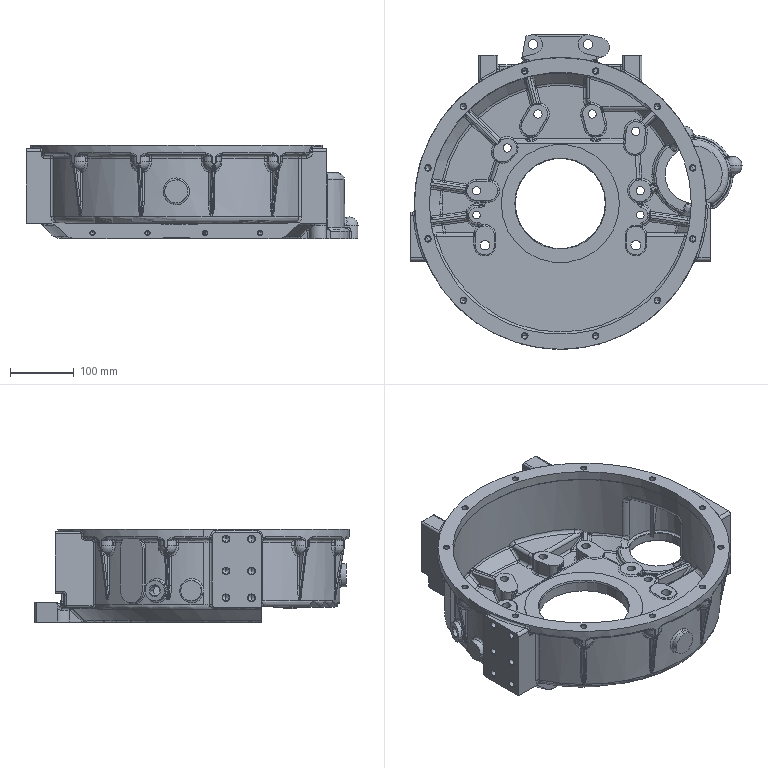Part | SolidWorks | features BaseBody 12 | 12 solids | 1872 faces | box 519.065 x 492 x 146 mm | volume 4296449 mm3 | cylinder 597 | spline 464 | torus 281 | plane 278 | cone 161 | sphere 91 | commonest cylinder face diameters 6 x182 10 x76 4 x65 8.5 x38 28 x35 30 x31